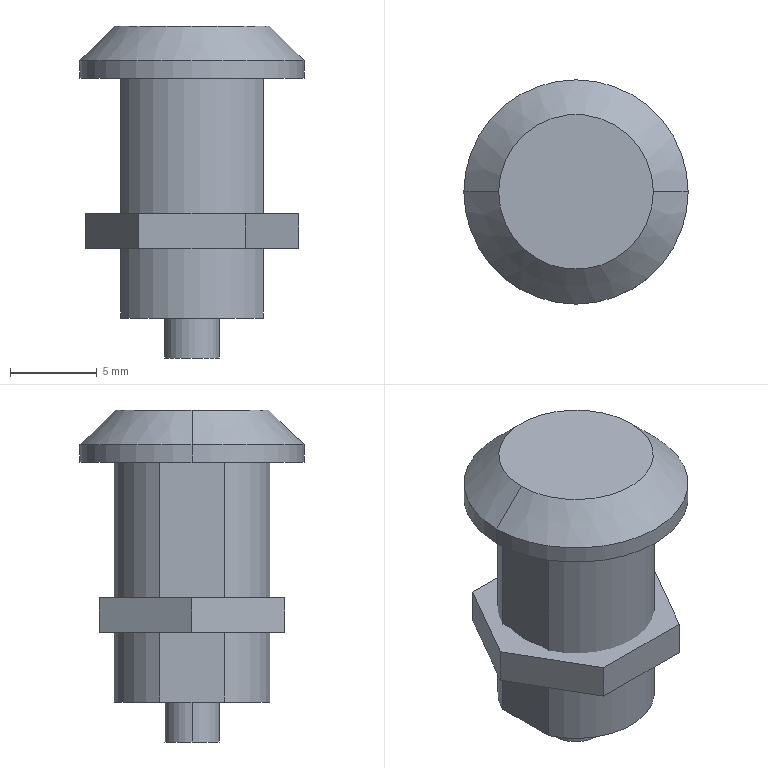Part | SolidWorks | features ICE 4, Chamfer 1, Extrusion 1 | 2 solids | 24 faces | box 12.9 x 12.9 x 19.1 mm | volume 1271 mm3 | plane 14 | cylinder 8 | cone 2 | commonest cylinder face diameters 3.16 x2 8.5 x2 9 x2 12.9 x2
STEP:
#1=CARTESIAN_POINT('',(-1.58,0.,-16.1));
#2=VERTEX_POINT('',#1);
#3=CARTESIAN_POINT('',(1.58,0.,-16.1));
#4=VERTEX_POINT('',#3);
#5=CARTESIAN_POINT('',(0.,0.,-16.1));
#6=DIRECTION('',(0.,0.,-1.));
#7=DIRECTION('',(-1.,0.,0.));
#8=AXIS2_PLACEMENT_3D('',#5,#6,#7);
#9=CIRCLE('',#8,1.58);
#10=EDGE_CURVE('',#2,#4,#9,.T.);
#11=ORIENTED_EDGE('',*,*,#10,.F.);
#12=CARTESIAN_POINT('',(-1.58,0.,-13.8));
#13=VERTEX_POINT('',#12);
#14=CARTESIAN_POINT('',(-1.58,0.,-16.1));
#15=DIRECTION('',(0.,0.,1.));
#16=VECTOR('',#15,1000.);
#17=LINE('',#14,#16);
#18=EDGE_CURVE('',#2,#13,#17,.T.);
#19=ORIENTED_EDGE('',*,*,#18,.T.);
#20=CARTESIAN_POINT('',(1.58,0.,-13.8));
#21=VERTEX_POINT('',#20);
#22=CARTESIAN_POINT('',(0.,0.,-13.8));
#23=DIRECTION('',(0.,0.,-1.));
#24=DIRECTION('',(-1.,0.,0.));
#25=AXIS2_PLACEMENT_3D('',#22,#23,#24);
#26=CIRCLE('',#25,1.58);
#27=EDGE_CURVE('',#13,#21,#26,.T.);
#28=ORIENTED_EDGE('',*,*,#27,.T.);
#29=CARTESIAN_POINT('',(1.58,0.,-16.1));
#30=DIRECTION('',(0.,0.,1.));
#31=VECTOR('',#30,1000.);
#32=LINE('',#29,#31);
#33=EDGE_CURVE('',#4,#21,#32,.T.);
#34=ORIENTED_EDGE('',*,*,#33,.F.);
#35=EDGE_LOOP('',(#11,#19,#28,#34));
#36=FACE_OUTER_BOUND('',#35,.T.);
#37=CARTESIAN_POINT('',(0.,0.,-16.1));
#38=DIRECTION('',(0.,0.,1.));
#39=DIRECTION('',(1.,0.,0.));
#40=AXIS2_PLACEMENT_3D('',#37,#38,#39);
#41=CYLINDRICAL_SURFACE('',#40,1.58);
#42=ADVANCED_FACE('',(#36),#41,.T.);
#43=CARTESIAN_POINT('',(4.45,0.,3.));
#44=VERTEX_POINT('',#43);
#45=CARTESIAN_POINT('',(-4.45,0.,3.));
#46=VERTEX_POINT('',#45);
#47=CARTESIAN_POINT('',(0.,0.,3.));
#48=DIRECTION('',(0.,0.,1.));
#49=DIRECTION('',(1.,0.,0.));
#50=AXIS2_PLACEMENT_3D('',#47,#48,#49);
#51=CIRCLE('',#50,4.45);
#52=EDGE_CURVE('',#44,#46,#51,.T.);
#53=ORIENTED_EDGE('',*,*,#52,.F.);
#54=CARTESIAN_POINT('',(6.45,0.,1.));
#55=VERTEX_POINT('',#54);
#56=CARTESIAN_POINT('',(4.45,0.,3.));
#57=DIRECTION('',(0.7071,0.,-0.7071));
#58=VECTOR('',#57,1000.);
#59=LINE('',#56,#58);
#60=EDGE_CURVE('',#44,#55,#59,.T.);
#61=ORIENTED_EDGE('',*,*,#60,.T.);
#62=CARTESIAN_POINT('',(-6.45,0.,1.));
#63=VERTEX_POINT('',#62);
#64=CARTESIAN_POINT('',(0.,0.,1.));
#65=DIRECTION('',(0.,0.,-1.));
#66=DIRECTION('',(1.,0.,0.));
#67=AXIS2_PLACEMENT_3D('',#64,#65,#66);
#68=CIRCLE('',#67,6.45);
#69=EDGE_CURVE('',#63,#55,#68,.T.);
#70=ORIENTED_EDGE('',*,*,#69,.F.);
#71=CARTESIAN_POINT('',(-4.45,0.,3.));
#72=DIRECTION('',(-0.7071,0.,-0.7071));
#73=VECTOR('',#72,1000.);
#74=LINE('',#71,#73);
#75=EDGE_CURVE('',#46,#63,#74,.T.);
#76=ORIENTED_EDGE('',*,*,#75,.F.);
#77=EDGE_LOOP('',(#53,#61,#70,#76));
#78=FACE_OUTER_BOUND('',#77,.T.);
#79=CARTESIAN_POINT('',(0.,0.,3.));
#80=DIRECTION('',(0.,0.,-1.));
#81=DIRECTION('',(-1.,0.,0.));
#82=AXIS2_PLACEMENT_3D('',#79,#80,#81);
#83=CONICAL_SURFACE('',#82,4.45,0.7854);
#84=ADVANCED_FACE('',(#78),#83,.T.);
#85=ORIENTED_EDGE('',*,*,#69,.T.);
#86=CARTESIAN_POINT('',(6.45,0.,0.));
#87=VERTEX_POINT('',#86);
#88=CARTESIAN_POINT('',(6.45,0.,3.));
#89=DIRECTION('',(0.,0.,-1.));
#90=VECTOR('',#89,1000.);
#91=LINE('',#88,#90);
#92=EDGE_CURVE('',#55,#87,#91,.T.);
#93=ORIENTED_EDGE('',*,*,#92,.T.);
#94=CARTESIAN_POINT('',(-6.45,0.,0.));
#95=VERTEX_POINT('',#94);
#96=CARTESIAN_POINT('',(0.,0.,0.));
#97=DIRECTION('',(0.,0.,1.));
#98=DIRECTION('',(1.,0.,0.));
#99=AXIS2_PLACEMENT_3D('',#96,#97,#98);
#100=CIRCLE('',#99,6.45);
#101=EDGE_CURVE('',#87,#95,#100,.T.);
#102=ORIENTED_EDGE('',*,*,#101,.T.);
#103=CARTESIAN_POINT('',(-6.45,0.,3.));
#104=DIRECTION('',(0.,0.,-1.));
#105=VECTOR('',#104,1000.);
#106=LINE('',#103,#105);
#107=EDGE_CURVE('',#63,#95,#106,.T.);
#108=ORIENTED_EDGE('',*,*,#107,.F.);
#109=EDGE_LOOP('',(#85,#93,#102,#108));
#110=FACE_OUTER_BOUND('',#109,.T.);
#111=CARTESIAN_POINT('',(0.,0.,3.));
#112=DIRECTION('',(0.,0.,-1.));
#113=DIRECTION('',(-1.,0.,0.));
#114=AXIS2_PLACEMENT_3D('',#111,#112,#113);
#115=CYLINDRICAL_SURFACE('',#114,6.45);
#116=ADVANCED_FACE('',(#110),#115,.T.);
#117=CARTESIAN_POINT('',(4.1,1.855,-13.8));
#118=VERTEX_POINT('',#117);
#119=CARTESIAN_POINT('',(4.1,1.855,0.));
#120=VERTEX_POINT('',#119);
#121=CARTESIAN_POINT('',(4.1,1.855,-13.8));
#122=DIRECTION('',(0.,0.,1.));
#123=VECTOR('',#122,1000.);
#124=LINE('',#121,#123);
#125=EDGE_CURVE('',#118,#120,#124,.T.);
#126=ORIENTED_EDGE('',*,*,#125,.F.);
#127=CARTESIAN_POINT('',(-4.1,1.855,-13.8));
#128=VERTEX_POINT('',#127);
#129=CARTESIAN_POINT('',(0.,0.,-13.8));
#130=DIRECTION('',(0.,0.,-1.));
#131=DIRECTION('',(-1.,0.,0.));
#132=AXIS2_PLACEMENT_3D('',#129,#130,#131);
#133=CIRCLE('',#132,4.5);
#134=EDGE_CURVE('',#128,#118,#133,.T.);
#135=ORIENTED_EDGE('',*,*,#134,.F.);
#136=CARTESIAN_POINT('',(-4.1,1.855,0.));
#137=VERTEX_POINT('',#136);
#138=CARTESIAN_POINT('',(-4.1,1.855,-13.8));
#139=DIRECTION('',(0.,0.,1.));
#140=VECTOR('',#139,1000.);
#141=LINE('',#138,#140);
#142=EDGE_CURVE('',#128,#137,#141,.T.);
#143=ORIENTED_EDGE('',*,*,#142,.T.);
#144=CARTESIAN_POINT('',(0.,0.,0.));
#145=DIRECTION('',(0.,0.,-1.));
#146=DIRECTION('',(-1.,0.,0.));
#147=AXIS2_PLACEMENT_3D('',#144,#145,#146);
#148=CIRCLE('',#147,4.5);
#149=EDGE_CURVE('',#137,#120,#148,.T.);
#150=ORIENTED_EDGE('',*,*,#149,.T.);
#151=EDGE_LOOP('',(#126,#135,#143,#150));
#152=FACE_OUTER_BOUND('',#151,.T.);
#153=CARTESIAN_POINT('',(0.,0.,-13.8));
#154=DIRECTION('',(0.,0.,1.));
#155=DIRECTION('',(1.,0.,0.));
#156=AXIS2_PLACEMENT_3D('',#153,#154,#155);
#157=CYLINDRICAL_SURFACE('',#156,4.5);
#158=ADVANCED_FACE('',(#152),#157,.T.);
#159=CARTESIAN_POINT('',(4.1,-1.855,0.));
#160=VERTEX_POINT('',#159);
#161=CARTESIAN_POINT('',(4.1,-1.855,-13.8));
#162=VERTEX_POINT('',#161);
#163=CARTESIAN_POINT('',(4.1,-1.855,-13.8));
#164=DIRECTION('',(0.,0.,-1.));
#165=VECTOR('',#164,1000.);
#166=LINE('',#163,#165);
#167=EDGE_CURVE('',#160,#162,#166,.T.);
#168=ORIENTED_EDGE('',*,*,#167,.F.);
#169=CARTESIAN_POINT('',(-4.1,-1.855,0.));
#170=VERTEX_POINT('',#169);
#171=CARTESIAN_POINT('',(0.,0.,0.));
#172=DIRECTION('',(0.,0.,-1.));
#173=DIRECTION('',(-1.,0.,0.));
#174=AXIS2_PLACEMENT_3D('',#171,#172,#173);
#175=CIRCLE('',#174,4.5);
#176=EDGE_CURVE('',#160,#170,#175,.T.);
#177=ORIENTED_EDGE('',*,*,#176,.T.);
#178=CARTESIAN_POINT('',(-4.1,-1.855,-13.8));
#179=VERTEX_POINT('',#178);
#180=CARTESIAN_POINT('',(-4.1,-1.855,-13.8));
#181=DIRECTION('',(0.,0.,-1.));
#182=VECTOR('',#181,1000.);
#183=LINE('',#180,#182);
#184=EDGE_CURVE('',#170,#179,#183,.T.);
#185=ORIENTED_EDGE('',*,*,#184,.T.);
#186=CARTESIAN_POINT('',(0.,0.,-13.8));
#187=DIRECTION('',(0.,0.,-1.));
#188=DIRECTION('',(-1.,0.,0.));
#189=AXIS2_PLACEMENT_3D('',#186,#187,#188);
#190=CIRCLE('',#189,4.5);
#191=EDGE_CURVE('',#162,#179,#190,.T.);
#192=ORIENTED_EDGE('',*,*,#191,.F.);
#193=EDGE_LOOP('',(#168,#177,#185,#192));
#194=FACE_OUTER_BOUND('',#193,.T.);
#195=CARTESIAN_POINT('',(0.,0.,-13.8));
#196=DIRECTION('',(0.,0.,1.));
#197=DIRECTION('',(1.,0.,0.));
#198=AXIS2_PLACEMENT_3D('',#195,#196,#197);
#199=CYLINDRICAL_SURFACE('',#198,4.5);
#200=ADVANCED_FACE('',(#194),#199,.T.);
#201=CARTESIAN_POINT('',(0.,0.,-13.8));
#202=DIRECTION('',(0.,0.,-1.));
#203=DIRECTION('',(-1.,0.,0.));
#204=AXIS2_PLACEMENT_3D('',#201,#202,#203);
#205=CIRCLE('',#204,1.58);
#206=EDGE_CURVE('',#21,#13,#205,.T.);
#207=ORIENTED_EDGE('',*,*,#206,.F.);
#208=ORIENTED_EDGE('',*,*,#27,.F.);
#209=EDGE_LOOP('',(#207,#208));
#210=FACE_BOUND('',#209,.T.);
#211=ORIENTED_EDGE('',*,*,#134,.T.);
#212=CARTESIAN_POINT('',(4.1,0.,-13.8));
#213=DIRECTION('',(0.,-1.,0.));
#214=VECTOR('',#213,1000.);
#215=LINE('',#212,#214);
#216=EDGE_CURVE('',#118,#162,#215,.T.);
#217=ORIENTED_EDGE('',*,*,#216,.T.);
#218=ORIENTED_EDGE('',*,*,#191,.T.);
#219=CARTESIAN_POINT('',(-4.1,0.,-13.8));
#220=DIRECTION('',(0.,-1.,0.));
#221=VECTOR('',#220,1000.);
#222=LINE('',#219,#221);
#223=EDGE_CURVE('',#128,#179,#222,.T.);
#224=ORIENTED_EDGE('',*,*,#223,.F.);
#225=EDGE_LOOP('',(#211,#217,#218,#224));
#226=FACE_OUTER_BOUND('',#225,.T.);
#227=CARTESIAN_POINT('',(0.,0.,-13.8));
#228=DIRECTION('',(0.,0.,-1.));
#229=DIRECTION('',(-1.,0.,0.));
#230=AXIS2_PLACEMENT_3D('',#227,#228,#229);
#231=PLANE('',#230);
#232=ADVANCED_FACE('',(#210,#226),#231,.T.);
#233=ORIENTED_EDGE('',*,*,#92,.F.);
#234=CARTESIAN_POINT('',(0.,0.,1.));
#235=DIRECTION('',(0.,0.,-1.));
#236=DIRECTION('',(1.,0.,0.));
#237=AXIS2_PLACEMENT_3D('',#234,#235,#236);
#238=CIRCLE('',#237,6.45);
#239=EDGE_CURVE('',#55,#63,#238,.T.);
#240=ORIENTED_EDGE('',*,*,#239,.T.);
#241=ORIENTED_EDGE('',*,*,#107,.T.);
#242=CARTESIAN_POINT('',(0.,0.,0.));
#243=DIRECTION('',(0.,0.,1.));
#244=DIRECTION('',(1.,0.,0.));
#245=AXIS2_PLACEMENT_3D('',#242,#243,#244);
#246=CIRCLE('',#245,6.45);
#247=EDGE_CURVE('',#95,#87,#246,.T.);
#248=ORIENTED_EDGE('',*,*,#247,.T.);
#249=EDGE_LOOP('',(#233,#240,#241,#248));
#250=FACE_OUTER_BOUND('',#249,.T.);
#251=CARTESIAN_POINT('',(0.,0.,3.));
#252=DIRECTION('',(0.,0.,-1.));
#253=DIRECTION('',(-1.,0.,0.));
#254=AXIS2_PLACEMENT_3D('',#251,#252,#253);
#255=CYLINDRICAL_SURFACE('',#254,6.45);
#256=ADVANCED_FACE('',(#250),#255,.T.);
#257=CARTESIAN_POINT('',(0.,0.,3.));
#258=DIRECTION('',(0.,0.,1.));
#259=DIRECTION('',(1.,0.,0.));
#260=AXIS2_PLACEMENT_3D('',#257,#258,#259);
#261=CIRCLE('',#260,4.45);
#262=EDGE_CURVE('',#46,#44,#261,.T.);
#263=ORIENTED_EDGE('',*,*,#262,.T.);
#264=ORIENTED_EDGE('',*,*,#52,.T.);
#265=EDGE_LOOP('',(#263,#264));
#266=FACE_OUTER_BOUND('',#265,.T.);
#267=CARTESIAN_POINT('',(0.,0.,3.));
#268=DIRECTION('',(0.,0.,1.));
#269=DIRECTION('',(1.,0.,0.));
#270=AXIS2_PLACEMENT_3D('',#267,#268,#269);
#271=PLANE('',#270);
#272=ADVANCED_FACE('',(#266),#271,.T.);
#273=ORIENTED_EDGE('',*,*,#176,.F.);
#274=CARTESIAN_POINT('',(4.1,-6.516,0.));
#275=DIRECTION('',(0.,1.,0.));
#276=VECTOR('',#275,1000.);
#277=LINE('',#274,#276);
#278=EDGE_CURVE('',#160,#120,#277,.T.);
#279=ORIENTED_EDGE('',*,*,#278,.T.);
#280=ORIENTED_EDGE('',*,*,#149,.F.);
#281=CARTESIAN_POINT('',(-4.1,-6.516,0.));
#282=DIRECTION('',(0.,1.,0.));
#283=VECTOR('',#282,1000.);
#284=LINE('',#281,#283);
#285=EDGE_CURVE('',#170,#137,#284,.T.);
#286=ORIENTED_EDGE('',*,*,#285,.F.);
#287=EDGE_LOOP('',(#273,#279,#280,#286));
#288=FACE_BOUND('',#287,.T.);
#289=ORIENTED_EDGE('',*,*,#247,.F.);
#290=ORIENTED_EDGE('',*,*,#101,.F.);
#291=EDGE_LOOP('',(#289,#290));
#292=FACE_OUTER_BOUND('',#291,.T.);
#293=CARTESIAN_POINT('',(0.,0.,0.));
#294=DIRECTION('',(0.,0.,1.));
#295=DIRECTION('',(1.,0.,0.));
#296=AXIS2_PLACEMENT_3D('',#293,#294,#295);
#297=PLANE('',#296);
#298=ADVANCED_FACE('',(#288,#292),#297,.F.);
#299=ORIENTED_EDGE('',*,*,#60,.F.);
#300=ORIENTED_EDGE('',*,*,#262,.F.);
#301=ORIENTED_EDGE('',*,*,#75,.T.);
#302=ORIENTED_EDGE('',*,*,#239,.F.);
#303=EDGE_LOOP('',(#299,#300,#301,#302));
#304=FACE_OUTER_BOUND('',#303,.T.);
#305=CARTESIAN_POINT('',(0.,0.,3.));
#306=DIRECTION('',(0.,0.,-1.));
#307=DIRECTION('',(-1.,0.,0.));
#308=AXIS2_PLACEMENT_3D('',#305,#306,#307);
#309=CONICAL_SURFACE('',#308,4.45,0.7854);
#310=ADVANCED_FACE('',(#304),#309,.T.);
#311=ORIENTED_EDGE('',*,*,#18,.F.);
#312=CARTESIAN_POINT('',(0.,0.,-16.1));
#313=DIRECTION('',(0.,0.,-1.));
#314=DIRECTION('',(-1.,0.,0.));
#315=AXIS2_PLACEMENT_3D('',#312,#313,#314);
#316=CIRCLE('',#315,1.58);
#317=EDGE_CURVE('',#4,#2,#316,.T.);
#318=ORIENTED_EDGE('',*,*,#317,.F.);
#319=ORIENTED_EDGE('',*,*,#33,.T.);
#320=ORIENTED_EDGE('',*,*,#206,.T.);
#321=EDGE_LOOP('',(#311,#318,#319,#320));
#322=FACE_OUTER_BOUND('',#321,.T.);
#323=CARTESIAN_POINT('',(0.,0.,-16.1));
#324=DIRECTION('',(0.,0.,1.));
#325=DIRECTION('',(1.,0.,0.));
#326=AXIS2_PLACEMENT_3D('',#323,#324,#325);
#327=CYLINDRICAL_SURFACE('',#326,1.58);
#328=ADVANCED_FACE('',(#322),#327,.T.);
#329=ORIENTED_EDGE('',*,*,#317,.T.);
#330=ORIENTED_EDGE('',*,*,#10,.T.);
#331=EDGE_LOOP('',(#329,#330));
#332=FACE_OUTER_BOUND('',#331,.T.);
#333=CARTESIAN_POINT('',(0.,0.,-16.1));
#334=DIRECTION('',(0.,0.,-1.));
#335=DIRECTION('',(-1.,0.,0.));
#336=AXIS2_PLACEMENT_3D('',#333,#334,#335);
#337=PLANE('',#336);
#338=ADVANCED_FACE('',(#332),#337,.T.);
#339=ORIENTED_EDGE('',*,*,#223,.T.);
#340=ORIENTED_EDGE('',*,*,#184,.F.);
#341=ORIENTED_EDGE('',*,*,#285,.T.);
#342=ORIENTED_EDGE('',*,*,#142,.F.);
#343=EDGE_LOOP('',(#339,#340,#341,#342));
#344=FACE_OUTER_BOUND('',#343,.T.);
#345=CARTESIAN_POINT('',(-4.1,-6.516,-15.));
#346=DIRECTION('',(1.,0.,0.));
#347=DIRECTION('',(0.,0.,-1.));
#348=AXIS2_PLACEMENT_3D('',#345,#346,#347);
#349=PLANE('',#348);
#350=ADVANCED_FACE('',(#344),#349,.F.);
#351=ORIENTED_EDGE('',*,*,#125,.T.);
#352=ORIENTED_EDGE('',*,*,#278,.F.);
#353=ORIENTED_EDGE('',*,*,#167,.T.);
#354=ORIENTED_EDGE('',*,*,#216,.F.);
#355=EDGE_LOOP('',(#351,#352,#353,#354));
#356=FACE_OUTER_BOUND('',#355,.T.);
#357=CARTESIAN_POINT('',(4.1,-6.516,-15.));
#358=DIRECTION('',(1.,0.,0.));
#359=DIRECTION('',(0.,0.,-1.));
#360=AXIS2_PLACEMENT_3D('',#357,#358,#359);
#361=PLANE('',#360);
#362=ADVANCED_FACE('',(#356),#361,.T.);
#363=CLOSED_SHELL('',(#42,#84,#116,#158,#200,#232,#256,#272,#298,#310,#328,#338,#350,#362));
#364=MANIFOLD_SOLID_BREP('',#363);
#365=CARTESIAN_POINT('',(4.25,0.,-9.8));
#366=VERTEX_POINT('',#365);
#367=CARTESIAN_POINT('',(-4.25,0.,-9.8));
#368=VERTEX_POINT('',#367);
#369=CARTESIAN_POINT('',(0.,0.,-9.8));
#370=DIRECTION('',(0.,0.,-1.));
#371=DIRECTION('',(-1.,0.,0.));
#372=AXIS2_PLACEMENT_3D('',#369,#370,#371);
#373=CIRCLE('',#372,4.25);
#374=EDGE_CURVE('',#366,#368,#373,.T.);
#375=ORIENTED_EDGE('',*,*,#374,.T.);
#376=CARTESIAN_POINT('',(-4.25,0.,-7.8));
#377=VERTEX_POINT('',#376);
#378=CARTESIAN_POINT('',(-4.25,0.,-9.8));
#379=DIRECTION('',(0.,0.,1.));
#380=VECTOR('',#379,1000.);
#381=LINE('',#378,#380);
#382=EDGE_CURVE('',#368,#377,#381,.T.);
#383=ORIENTED_EDGE('',*,*,#382,.T.);
#384=CARTESIAN_POINT('',(4.25,0.,-7.8));
#385=VERTEX_POINT('',#384);
#386=CARTESIAN_POINT('',(0.,0.,-7.8));
#387=DIRECTION('',(0.,0.,-1.));
#388=DIRECTION('',(-1.,0.,0.));
#389=AXIS2_PLACEMENT_3D('',#386,#387,#388);
#390=CIRCLE('',#389,4.25);
#391=EDGE_CURVE('',#385,#377,#390,.T.);
#392=ORIENTED_EDGE('',*,*,#391,.F.);
#393=CARTESIAN_POINT('',(4.25,0.,-9.8));
#394=DIRECTION('',(0.,0.,1.));
#395=VECTOR('',#394,1000.);
#396=LINE('',#393,#395);
#397=EDGE_CURVE('',#366,#385,#396,.T.);
#398=ORIENTED_EDGE('',*,*,#397,.F.);
#399=EDGE_LOOP('',(#375,#383,#392,#398));
#400=FACE_OUTER_BOUND('',#399,.T.);
#401=CARTESIAN_POINT('',(0.,0.,-9.8));
#402=DIRECTION('',(0.,0.,1.));
#403=DIRECTION('',(1.,0.,0.));
#404=AXIS2_PLACEMENT_3D('',#401,#402,#403);
#405=CYLINDRICAL_SURFACE('',#404,4.25);
#406=ADVANCED_FACE('',(#400),#405,.F.);
#407=CARTESIAN_POINT('',(-3.075,5.326,-9.8));
#408=VERTEX_POINT('',#407);
#409=CARTESIAN_POINT('',(3.075,5.326,-9.8));
#410=VERTEX_POINT('',#409);
#411=CARTESIAN_POINT('',(-3.075,5.326,-9.8));
#412=DIRECTION('',(1.,0.,0.));
#413=VECTOR('',#412,1000.);
#414=LINE('',#411,#413);
#415=EDGE_CURVE('',#408,#410,#414,.T.);
#416=ORIENTED_EDGE('',*,*,#415,.T.);
#417=CARTESIAN_POINT('',(6.15,0.,-9.8));
#418=VERTEX_POINT('',#417);
#419=CARTESIAN_POINT('',(3.075,5.326,-9.8));
#420=DIRECTION('',(0.5,-0.866,0.));
#421=VECTOR('',#420,1000.);
#422=LINE('',#419,#421);
#423=EDGE_CURVE('',#410,#418,#422,.T.);
#424=ORIENTED_EDGE('',*,*,#423,.T.);
#425=CARTESIAN_POINT('',(3.075,-5.326,-9.8));
#426=VERTEX_POINT('',#425);
#427=CARTESIAN_POINT('',(6.15,0.,-9.8));
#428=DIRECTION('',(-0.5,-0.866,0.));
#429=VECTOR('',#428,1000.);
#430=LINE('',#427,#429);
#431=EDGE_CURVE('',#418,#426,#430,.T.);
#432=ORIENTED_EDGE('',*,*,#431,.T.);
#433=CARTESIAN_POINT('',(-3.075,-5.326,-9.8));
#434=VERTEX_POINT('',#433);
#435=CARTESIAN_POINT('',(3.075,-5.326,-9.8));
#436=DIRECTION('',(-1.,0.,0.));
#437=VECTOR('',#436,1000.);
#438=LINE('',#435,#437);
#439=EDGE_CURVE('',#426,#434,#438,.T.);
#440=ORIENTED_EDGE('',*,*,#439,.T.);
#441=CARTESIAN_POINT('',(-6.15,0.,-9.8));
#442=VERTEX_POINT('',#441);
#443=CARTESIAN_POINT('',(-3.075,-5.326,-9.8));
#444=DIRECTION('',(-0.5,0.866,0.));
#445=VECTOR('',#444,1000.);
#446=LINE('',#443,#445);
#447=EDGE_CURVE('',#434,#442,#446,.T.);
#448=ORIENTED_EDGE('',*,*,#447,.T.);
#449=CARTESIAN_POINT('',(-6.15,0.,-9.8));
#450=DIRECTION('',(0.5,0.866,0.));
#451=VECTOR('',#450,1000.);
#452=LINE('',#449,#451);
#453=EDGE_CURVE('',#442,#408,#452,.T.);
#454=ORIENTED_EDGE('',*,*,#453,.T.);
#455=EDGE_LOOP('',(#416,#424,#432,#440,#448,#454));
#456=FACE_OUTER_BOUND('',#455,.T.);
#457=ORIENTED_EDGE('',*,*,#374,.F.);
#458=CARTESIAN_POINT('',(0.,0.,-9.8));
#459=DIRECTION('',(0.,0.,-1.));
#460=DIRECTION('',(-1.,0.,0.));
#461=AXIS2_PLACEMENT_3D('',#458,#459,#460);
#462=CIRCLE('',#461,4.25);
#463=EDGE_CURVE('',#368,#366,#462,.T.);
#464=ORIENTED_EDGE('',*,*,#463,.F.);
#465=EDGE_LOOP('',(#457,#464));
#466=FACE_BOUND('',#465,.T.);
#467=CARTESIAN_POINT('',(0.,0.,-9.8));
#468=DIRECTION('',(0.,0.,-1.));
#469=DIRECTION('',(-1.,0.,0.));
#470=AXIS2_PLACEMENT_3D('',#467,#468,#469);
#471=PLANE('',#470);
#472=ADVANCED_FACE('',(#456,#466),#471,.T.);
#473=CARTESIAN_POINT('',(-3.075,5.326,-7.8));
#474=VERTEX_POINT('',#473);
#475=CARTESIAN_POINT('',(3.075,5.326,-7.8));
#476=VERTEX_POINT('',#475);
#477=CARTESIAN_POINT('',(-3.075,5.326,-7.8));
#478=DIRECTION('',(1.,0.,0.));
#479=VECTOR('',#478,1000.);
#480=LINE('',#477,#479);
#481=EDGE_CURVE('',#474,#476,#480,.T.);
#482=ORIENTED_EDGE('',*,*,#481,.F.);
#483=CARTESIAN_POINT('',(-6.15,0.,-7.8));
#484=VERTEX_POINT('',#483);
#485=CARTESIAN_POINT('',(-6.15,0.,-7.8));
#486=DIRECTION('',(0.5,0.866,0.));
#487=VECTOR('',#486,1000.);
#488=LINE('',#485,#487);
#489=EDGE_CURVE('',#484,#474,#488,.T.);
#490=ORIENTED_EDGE('',*,*,#489,.F.);
#491=CARTESIAN_POINT('',(-3.075,-5.326,-7.8));
#492=VERTEX_POINT('',#491);
#493=CARTESIAN_POINT('',(-3.075,-5.326,-7.8));
#494=DIRECTION('',(-0.5,0.866,0.));
#495=VECTOR('',#494,1000.);
#496=LINE('',#493,#495);
#497=EDGE_CURVE('',#492,#484,#496,.T.);
#498=ORIENTED_EDGE('',*,*,#497,.F.);
#499=CARTESIAN_POINT('',(3.075,-5.326,-7.8));
#500=VERTEX_POINT('',#499);
#501=CARTESIAN_POINT('',(3.075,-5.326,-7.8));
#502=DIRECTION('',(-1.,0.,0.));
#503=VECTOR('',#502,1000.);
#504=LINE('',#501,#503);
#505=EDGE_CURVE('',#500,#492,#504,.T.);
#506=ORIENTED_EDGE('',*,*,#505,.F.);
#507=CARTESIAN_POINT('',(6.15,0.,-7.8));
#508=VERTEX_POINT('',#507);
#509=CARTESIAN_POINT('',(6.15,0.,-7.8));
#510=DIRECTION('',(-0.5,-0.866,0.));
#511=VECTOR('',#510,1000.);
#512=LINE('',#509,#511);
#513=EDGE_CURVE('',#508,#500,#512,.T.);
#514=ORIENTED_EDGE('',*,*,#513,.F.);
#515=CARTESIAN_POINT('',(3.075,5.326,-7.8));
#516=DIRECTION('',(0.5,-0.866,0.));
#517=VECTOR('',#516,1000.);
#518=LINE('',#515,#517);
#519=EDGE_CURVE('',#476,#508,#518,.T.);
#520=ORIENTED_EDGE('',*,*,#519,.F.);
#521=EDGE_LOOP('',(#482,#490,#498,#506,#514,#520));
#522=FACE_OUTER_BOUND('',#521,.T.);
#523=ORIENTED_EDGE('',*,*,#391,.T.);
#524=CARTESIAN_POINT('',(0.,0.,-7.8));
#525=DIRECTION('',(0.,0.,-1.));
#526=DIRECTION('',(-1.,0.,0.));
#527=AXIS2_PLACEMENT_3D('',#524,#525,#526);
#528=CIRCLE('',#527,4.25);
#529=EDGE_CURVE('',#377,#385,#528,.T.);
#530=ORIENTED_EDGE('',*,*,#529,.T.);
#531=EDGE_LOOP('',(#523,#530));
#532=FACE_BOUND('',#531,.T.);
#533=CARTESIAN_POINT('',(0.,0.,-7.8));
#534=DIRECTION('',(0.,0.,-1.));
#535=DIRECTION('',(-1.,0.,0.));
#536=AXIS2_PLACEMENT_3D('',#533,#534,#535);
#537=PLANE('',#536);
#538=ADVANCED_FACE('',(#522,#532),#537,.F.);
#539=ORIENTED_EDGE('',*,*,#481,.T.);
#540=CARTESIAN_POINT('',(3.075,5.326,-9.8));
#541=DIRECTION('',(0.,0.,1.));
#542=VECTOR('',#541,1000.);
#543=LINE('',#540,#542);
#544=EDGE_CURVE('',#410,#476,#543,.T.);
#545=ORIENTED_EDGE('',*,*,#544,.F.);
#546=ORIENTED_EDGE('',*,*,#415,.F.);
#547=CARTESIAN_POINT('',(-3.075,5.326,-9.8));
#548=DIRECTION('',(0.,0.,1.));
#549=VECTOR('',#548,1000.);
#550=LINE('',#547,#549);
#551=EDGE_CURVE('',#408,#474,#550,.T.);
#552=ORIENTED_EDGE('',*,*,#551,.T.);
#553=EDGE_LOOP('',(#539,#545,#546,#552));
#554=FACE_OUTER_BOUND('',#553,.T.);
#555=CARTESIAN_POINT('',(-3.075,5.326,-9.8));
#556=DIRECTION('',(0.,-1.,0.));
#557=DIRECTION('',(0.,0.,-1.));
#558=AXIS2_PLACEMENT_3D('',#555,#556,#557);
#559=PLANE('',#558);
#560=ADVANCED_FACE('',(#554),#559,.F.);
#561=ORIENTED_EDGE('',*,*,#519,.T.);
#562=CARTESIAN_POINT('',(6.15,0.,-9.8));
#563=DIRECTION('',(0.,0.,1.));
#564=VECTOR('',#563,1000.);
#565=LINE('',#562,#564);
#566=EDGE_CURVE('',#418,#508,#565,.T.);
#567=ORIENTED_EDGE('',*,*,#566,.F.);
#568=ORIENTED_EDGE('',*,*,#423,.F.);
#569=ORIENTED_EDGE('',*,*,#544,.T.);
#570=EDGE_LOOP('',(#561,#567,#568,#569));
#571=FACE_OUTER_BOUND('',#570,.T.);
#572=CARTESIAN_POINT('',(3.075,5.326,-9.8));
#573=DIRECTION('',(-0.866,-0.5,0.));
#574=DIRECTION('',(0.5,-0.866,0.));
#575=AXIS2_PLACEMENT_3D('',#572,#573,#574);
#576=PLANE('',#575);
#577=ADVANCED_FACE('',(#571),#576,.F.);
#578=ORIENTED_EDGE('',*,*,#513,.T.);
#579=CARTESIAN_POINT('',(3.075,-5.326,-9.8));
#580=DIRECTION('',(0.,0.,1.));
#581=VECTOR('',#580,1000.);
#582=LINE('',#579,#581);
#583=EDGE_CURVE('',#426,#500,#582,.T.);
#584=ORIENTED_EDGE('',*,*,#583,.F.);
#585=ORIENTED_EDGE('',*,*,#431,.F.);
#586=ORIENTED_EDGE('',*,*,#566,.T.);
#587=EDGE_LOOP('',(#578,#584,#585,#586));
#588=FACE_OUTER_BOUND('',#587,.T.);
#589=CARTESIAN_POINT('',(6.15,0.,-9.8));
#590=DIRECTION('',(-0.866,0.5,0.));
#591=DIRECTION('',(-0.5,-0.866,0.));
#592=AXIS2_PLACEMENT_3D('',#589,#590,#591);
#593=PLANE('',#592);
#594=ADVANCED_FACE('',(#588),#593,.F.);
#595=ORIENTED_EDGE('',*,*,#505,.T.);
#596=CARTESIAN_POINT('',(-3.075,-5.326,-9.8));
#597=DIRECTION('',(0.,0.,1.));
#598=VECTOR('',#597,1000.);
#599=LINE('',#596,#598);
#600=EDGE_CURVE('',#434,#492,#599,.T.);
#601=ORIENTED_EDGE('',*,*,#600,.F.);
#602=ORIENTED_EDGE('',*,*,#439,.F.);
#603=ORIENTED_EDGE('',*,*,#583,.T.);
#604=EDGE_LOOP('',(#595,#601,#602,#603));
#605=FACE_OUTER_BOUND('',#604,.T.);
#606=CARTESIAN_POINT('',(3.075,-5.326,-9.8));
#607=DIRECTION('',(0.,1.,0.));
#608=DIRECTION('',(-1.,0.,0.));
#609=AXIS2_PLACEMENT_3D('',#606,#607,#608);
#610=PLANE('',#609);
#611=ADVANCED_FACE('',(#605),#610,.F.);
#612=ORIENTED_EDGE('',*,*,#497,.T.);
#613=CARTESIAN_POINT('',(-6.15,0.,-9.8));
#614=DIRECTION('',(0.,0.,1.));
#615=VECTOR('',#614,1000.);
#616=LINE('',#613,#615);
#617=EDGE_CURVE('',#442,#484,#616,.T.);
#618=ORIENTED_EDGE('',*,*,#617,.F.);
#619=ORIENTED_EDGE('',*,*,#447,.F.);
#620=ORIENTED_EDGE('',*,*,#600,.T.);
#621=EDGE_LOOP('',(#612,#618,#619,#620));
#622=FACE_OUTER_BOUND('',#621,.T.);
#623=CARTESIAN_POINT('',(-3.075,-5.326,-9.8));
#624=DIRECTION('',(0.866,0.5,0.));
#625=DIRECTION('',(-0.5,0.866,0.));
#626=AXIS2_PLACEMENT_3D('',#623,#624,#625);
#627=PLANE('',#626);
#628=ADVANCED_FACE('',(#622),#627,.F.);
#629=ORIENTED_EDGE('',*,*,#489,.T.);
#630=ORIENTED_EDGE('',*,*,#551,.F.);
#631=ORIENTED_EDGE('',*,*,#453,.F.);
#632=ORIENTED_EDGE('',*,*,#617,.T.);
#633=EDGE_LOOP('',(#629,#630,#631,#632));
#634=FACE_OUTER_BOUND('',#633,.T.);
#635=CARTESIAN_POINT('',(-6.15,0.,-9.8));
#636=DIRECTION('',(0.866,-0.5,0.));
#637=DIRECTION('',(0.5,0.866,0.));
#638=AXIS2_PLACEMENT_3D('',#635,#636,#637);
#639=PLANE('',#638);
#640=ADVANCED_FACE('',(#634),#639,.F.);
#641=ORIENTED_EDGE('',*,*,#382,.F.);
#642=ORIENTED_EDGE('',*,*,#463,.T.);
#643=ORIENTED_EDGE('',*,*,#397,.T.);
#644=ORIENTED_EDGE('',*,*,#529,.F.);
#645=EDGE_LOOP('',(#641,#642,#643,#644));
#646=FACE_OUTER_BOUND('',#645,.T.);
#647=CARTESIAN_POINT('',(0.,0.,-9.8));
#648=DIRECTION('',(0.,0.,1.));
#649=DIRECTION('',(1.,0.,0.));
#650=AXIS2_PLACEMENT_3D('',#647,#648,#649);
#651=CYLINDRICAL_SURFACE('',#650,4.25);
#652=ADVANCED_FACE('',(#646),#651,.F.);
#653=CLOSED_SHELL('',(#406,#472,#538,#560,#577,#594,#611,#628,#640,#652));
#654=MANIFOLD_SOLID_BREP('',#653);
#655=CARTESIAN_POINT('',(0.,0.,0.));
#656=DIRECTION('',(0.,0.,1.));
#657=DIRECTION('',(1.,0.,0.));
#658=AXIS2_PLACEMENT_3D('',#655,#656,#657);
#659=(LENGTH_UNIT()NAMED_UNIT(*)SI_UNIT(.MILLI.,.METRE.));
#660=UNCERTAINTY_MEASURE_WITH_UNIT(LENGTH_MEASURE(0.00001),#659,'','');
#661=(NAMED_UNIT(*)PLANE_ANGLE_UNIT()SI_UNIT($,.RADIAN.));
#662=(NAMED_UNIT(*)SI_UNIT($,.STERADIAN.)SOLID_ANGLE_UNIT());
#663=(GEOMETRIC_REPRESENTATION_CONTEXT(3)GLOBAL_UNCERTAINTY_ASSIGNED_CONTEXT((#660))GLOBAL_UNIT_ASSIGNED_CONTEXT((#659,#661,#662))REPRESENTATION_CONTEXT('',''));
#664=ADVANCED_BREP_SHAPE_REPRESENTATION('',(#364,#654,#658),#663);